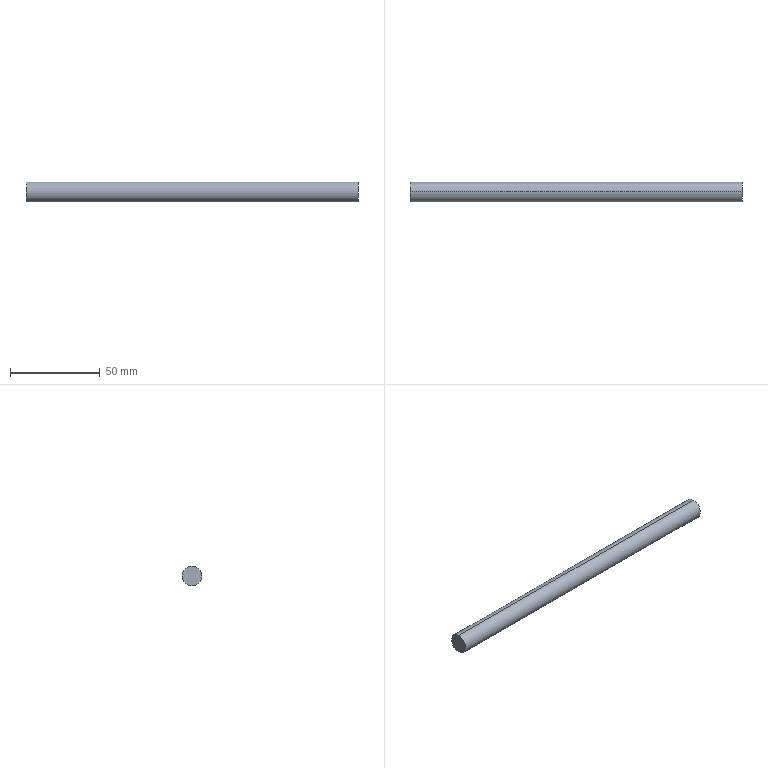Part | STEP file | 4-20.sldasm-Part-394 | 1 solid | 4 faces | box 185 x 11.11 x 11.11 mm | volume 17935 mm3 | cylinder 2 | plane 2 | commonest cylinder face diameters 11.11 x2
STEP:
#1=CARTESIAN_POINT('',(-55.,400.,179.555));
#2=VERTEX_POINT('',#1);
#3=CARTESIAN_POINT('',(-55.,400.,168.445));
#4=VERTEX_POINT('',#3);
#5=CARTESIAN_POINT('',(-55.,400.,174.));
#6=DIRECTION('',(1.,0.,0.));
#7=DIRECTION('',(0.,0.,1.));
#8=AXIS2_PLACEMENT_3D('',#5,#6,#7);
#9=CIRCLE('',#8,5.555);
#10=EDGE_CURVE('',#2,#4,#9,.T.);
#11=ORIENTED_EDGE('',*,*,#10,.T.);
#12=CARTESIAN_POINT('',(130.,400.,168.445));
#13=VERTEX_POINT('',#12);
#14=CARTESIAN_POINT('',(55.,400.,168.445));
#15=DIRECTION('',(1.,0.,0.));
#16=VECTOR('',#15,1000.);
#17=LINE('',#14,#16);
#18=EDGE_CURVE('',#4,#13,#17,.T.);
#19=ORIENTED_EDGE('',*,*,#18,.T.);
#20=CARTESIAN_POINT('',(130.,400.,179.555));
#21=VERTEX_POINT('',#20);
#22=CARTESIAN_POINT('',(130.,400.,174.));
#23=DIRECTION('',(-1.,0.,0.));
#24=DIRECTION('',(0.,0.,-1.));
#25=AXIS2_PLACEMENT_3D('',#22,#23,#24);
#26=CIRCLE('',#25,5.555);
#27=EDGE_CURVE('',#13,#21,#26,.T.);
#28=ORIENTED_EDGE('',*,*,#27,.T.);
#29=CARTESIAN_POINT('',(55.,400.,179.555));
#30=DIRECTION('',(1.,0.,0.));
#31=VECTOR('',#30,1000.);
#32=LINE('',#29,#31);
#33=EDGE_CURVE('',#2,#21,#32,.T.);
#34=ORIENTED_EDGE('',*,*,#33,.F.);
#35=EDGE_LOOP('',(#11,#19,#28,#34));
#36=FACE_OUTER_BOUND('',#35,.T.);
#37=CARTESIAN_POINT('',(55.,400.,174.));
#38=DIRECTION('',(1.,0.,0.));
#39=DIRECTION('',(0.,0.,1.));
#40=AXIS2_PLACEMENT_3D('',#37,#38,#39);
#41=CYLINDRICAL_SURFACE('',#40,5.555);
#42=ADVANCED_FACE('',(#36),#41,.T.);
#43=ORIENTED_EDGE('',*,*,#18,.F.);
#44=CARTESIAN_POINT('',(-55.,400.,174.));
#45=DIRECTION('',(1.,0.,0.));
#46=DIRECTION('',(0.,0.,1.));
#47=AXIS2_PLACEMENT_3D('',#44,#45,#46);
#48=CIRCLE('',#47,5.555);
#49=EDGE_CURVE('',#4,#2,#48,.T.);
#50=ORIENTED_EDGE('',*,*,#49,.T.);
#51=ORIENTED_EDGE('',*,*,#33,.T.);
#52=CARTESIAN_POINT('',(130.,400.,174.));
#53=DIRECTION('',(-1.,0.,0.));
#54=DIRECTION('',(0.,0.,-1.));
#55=AXIS2_PLACEMENT_3D('',#52,#53,#54);
#56=CIRCLE('',#55,5.555);
#57=EDGE_CURVE('',#21,#13,#56,.T.);
#58=ORIENTED_EDGE('',*,*,#57,.T.);
#59=EDGE_LOOP('',(#43,#50,#51,#58));
#60=FACE_OUTER_BOUND('',#59,.T.);
#61=CARTESIAN_POINT('',(55.,400.,174.));
#62=DIRECTION('',(1.,0.,0.));
#63=DIRECTION('',(0.,0.,1.));
#64=AXIS2_PLACEMENT_3D('',#61,#62,#63);
#65=CYLINDRICAL_SURFACE('',#64,5.555);
#66=ADVANCED_FACE('',(#60),#65,.T.);
#67=ORIENTED_EDGE('',*,*,#10,.F.);
#68=ORIENTED_EDGE('',*,*,#49,.F.);
#69=EDGE_LOOP('',(#67,#68));
#70=FACE_OUTER_BOUND('',#69,.T.);
#71=CARTESIAN_POINT('',(-55.,400.,174.));
#72=DIRECTION('',(-1.,0.,0.));
#73=DIRECTION('',(0.,0.,-1.));
#74=AXIS2_PLACEMENT_3D('',#71,#72,#73);
#75=PLANE('',#74);
#76=ADVANCED_FACE('',(#70),#75,.T.);
#77=ORIENTED_EDGE('',*,*,#57,.F.);
#78=ORIENTED_EDGE('',*,*,#27,.F.);
#79=EDGE_LOOP('',(#77,#78));
#80=FACE_OUTER_BOUND('',#79,.T.);
#81=CARTESIAN_POINT('',(130.,30.,374.));
#82=DIRECTION('',(1.,0.,0.));
#83=DIRECTION('',(0.,0.,-1.));
#84=AXIS2_PLACEMENT_3D('',#81,#82,#83);
#85=PLANE('',#84);
#86=ADVANCED_FACE('',(#80),#85,.T.);
#87=CLOSED_SHELL('',(#42,#66,#76,#86));
#88=MANIFOLD_SOLID_BREP('',#87);
#89=CARTESIAN_POINT('',(0.,0.,0.));
#90=DIRECTION('',(0.,0.,1.));
#91=DIRECTION('',(1.,0.,0.));
#92=AXIS2_PLACEMENT_3D('',#89,#90,#91);
#93=(LENGTH_UNIT()NAMED_UNIT(*)SI_UNIT(.MILLI.,.METRE.));
#94=UNCERTAINTY_MEASURE_WITH_UNIT(LENGTH_MEASURE(0.00001),#93,'','');
#95=(NAMED_UNIT(*)PLANE_ANGLE_UNIT()SI_UNIT($,.RADIAN.));
#96=(NAMED_UNIT(*)SI_UNIT($,.STERADIAN.)SOLID_ANGLE_UNIT());
#97=(GEOMETRIC_REPRESENTATION_CONTEXT(3)GLOBAL_UNCERTAINTY_ASSIGNED_CONTEXT((#94))GLOBAL_UNIT_ASSIGNED_CONTEXT((#93,#95,#96))REPRESENTATION_CONTEXT('',''));
#98=ADVANCED_BREP_SHAPE_REPRESENTATION('',(#88,#92),#97);